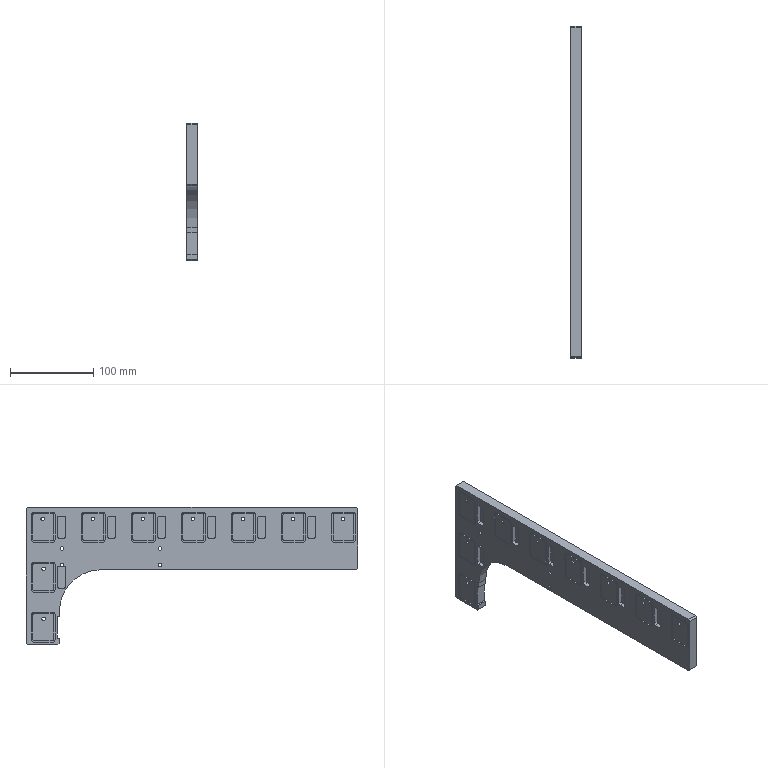Part | SolidWorks | features ICE 9, LPattern 7, HoleWzd 6, Fillet 4, Cut 3, Chamfer 2, Extrusion 1 | 1 solid | 270 faces | box 12 x 398 x 165 mm | volume 392950 mm3 | plane 143 | cylinder 127 | commonest cylinder face diameters 4.1 x36 7.7 x36 4 x28 4.2 x26 100 x1